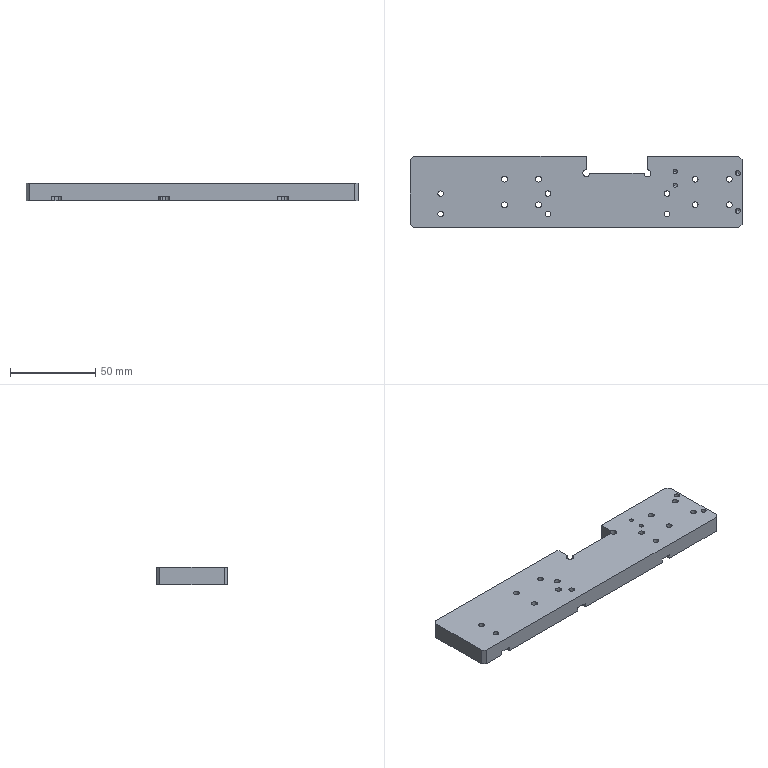Part | NX | features BREP 1 | 1 solid | 112 faces | box 195 x 42 x 10 mm | volume 73666 mm3 | cylinder 65 | plane 35 | cone 12 | commonest cylinder face diameters 3.4 x16 7 x16 3.3 x12 4 x9 2.5 x4 3 x4